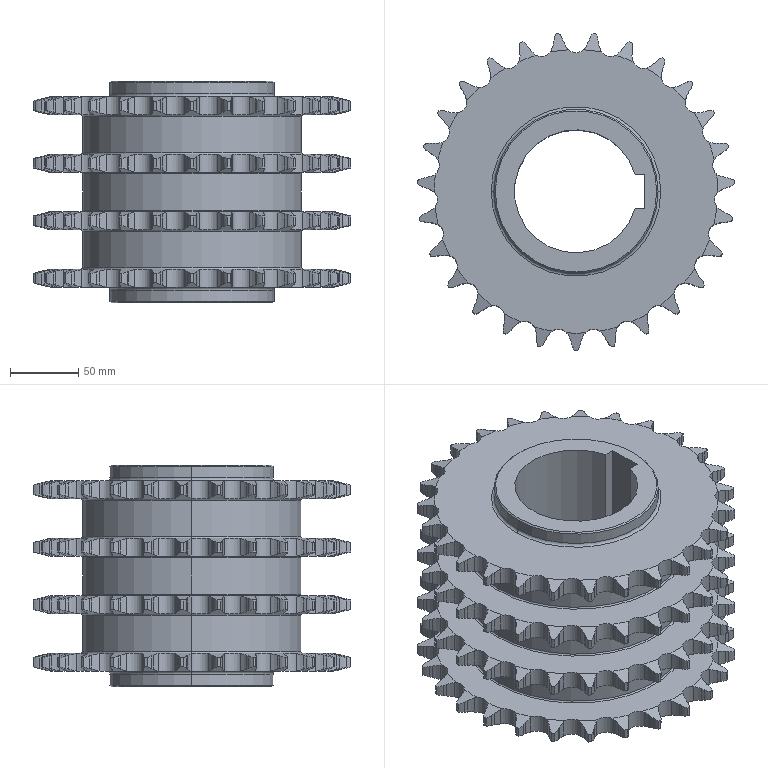Part | STEP file | 03-Main drive sprocket | 1 solid | 1132 faces | box 232.271 x 231.883 x 162 mm | volume 2819895 mm3 | cylinder 659 | plane 229 | cone 228 | torus 16 | commonest cylinder face diameters 26.077 x216 41.357 x216 15.957 x108 232.551 x108 160 x6 120 x4